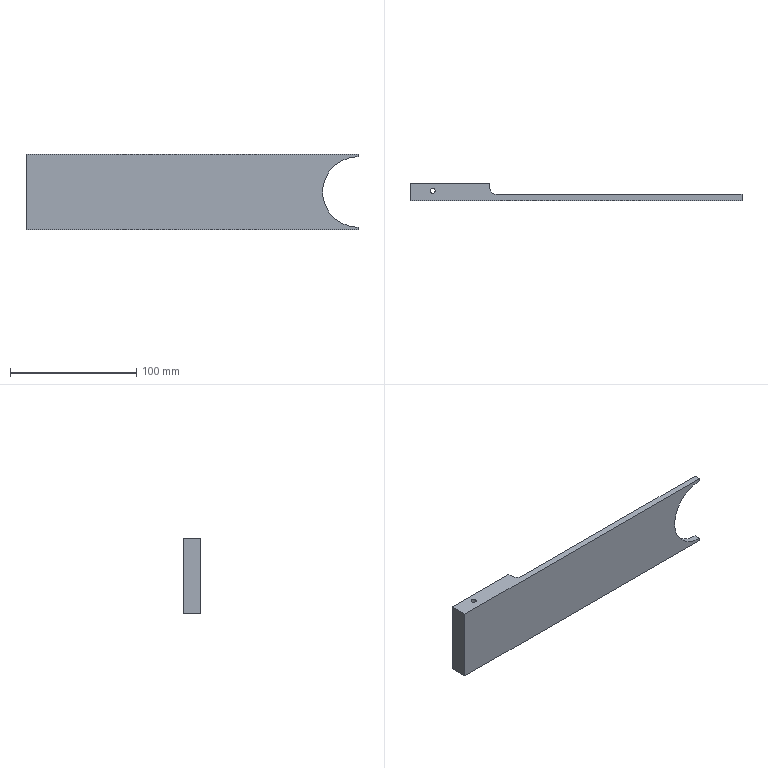Part | SolidWorks | features ICE 2, Extrusion 1, Fillet 1 | 1 solid | 13 faces | box 263.439 x 13.991 x 60 mm | volume 106666 mm3 | plane 9 | cylinder 4 | commonest cylinder face diameters 4 x2 10 x1 56 x1
STEP:
#1=CARTESIAN_POINT('',(-97.439,5.491,-30.));
#2=VERTEX_POINT('',#1);
#3=CARTESIAN_POINT('',(-93.439,5.491,-30.));
#4=VERTEX_POINT('',#3);
#5=CARTESIAN_POINT('',(-95.439,5.491,-30.));
#6=DIRECTION('',(0.,0.,1.));
#7=DIRECTION('',(1.,0.,0.));
#8=AXIS2_PLACEMENT_3D('',#5,#6,#7);
#9=CIRCLE('',#8,2.);
#10=EDGE_CURVE('',#2,#4,#9,.T.);
#11=ORIENTED_EDGE('',*,*,#10,.F.);
#12=CARTESIAN_POINT('',(-97.439,5.491,30.));
#13=VERTEX_POINT('',#12);
#14=CARTESIAN_POINT('',(-97.439,5.491,-30.));
#15=DIRECTION('',(0.,0.,1.));
#16=VECTOR('',#15,1000.);
#17=LINE('',#14,#16);
#18=EDGE_CURVE('',#2,#13,#17,.T.);
#19=ORIENTED_EDGE('',*,*,#18,.T.);
#20=CARTESIAN_POINT('',(-93.439,5.491,30.));
#21=VERTEX_POINT('',#20);
#22=CARTESIAN_POINT('',(-95.439,5.491,30.));
#23=DIRECTION('',(0.,0.,1.));
#24=DIRECTION('',(1.,0.,0.));
#25=AXIS2_PLACEMENT_3D('',#22,#23,#24);
#26=CIRCLE('',#25,2.);
#27=EDGE_CURVE('',#13,#21,#26,.T.);
#28=ORIENTED_EDGE('',*,*,#27,.T.);
#29=CARTESIAN_POINT('',(-93.439,5.491,-30.));
#30=DIRECTION('',(0.,0.,1.));
#31=VECTOR('',#30,1000.);
#32=LINE('',#29,#31);
#33=EDGE_CURVE('',#4,#21,#32,.T.);
#34=ORIENTED_EDGE('',*,*,#33,.F.);
#35=EDGE_LOOP('',(#11,#19,#28,#34));
#36=FACE_OUTER_BOUND('',#35,.T.);
#37=CARTESIAN_POINT('',(-95.439,5.491,-30.));
#38=DIRECTION('',(0.,0.,1.));
#39=DIRECTION('',(1.,0.,0.));
#40=AXIS2_PLACEMENT_3D('',#37,#38,#39);
#41=CYLINDRICAL_SURFACE('',#40,2.);
#42=ADVANCED_FACE('',(#36),#41,.F.);
#43=CARTESIAN_POINT('',(150.,-2.5,30.));
#44=VERTEX_POINT('',#43);
#45=CARTESIAN_POINT('',(150.,-2.5,28.));
#46=VERTEX_POINT('',#45);
#47=CARTESIAN_POINT('',(150.,-2.5,30.));
#48=DIRECTION('',(0.,0.,-1.));
#49=VECTOR('',#48,1000.);
#50=LINE('',#47,#49);
#51=EDGE_CURVE('',#44,#46,#50,.T.);
#52=ORIENTED_EDGE('',*,*,#51,.T.);
#53=CARTESIAN_POINT('',(150.,2.5,28.));
#54=VERTEX_POINT('',#53);
#55=CARTESIAN_POINT('',(150.,2.5,28.));
#56=DIRECTION('',(0.,-1.,0.));
#57=VECTOR('',#56,1000.);
#58=LINE('',#55,#57);
#59=EDGE_CURVE('',#54,#46,#58,.T.);
#60=ORIENTED_EDGE('',*,*,#59,.F.);
#61=CARTESIAN_POINT('',(150.,2.5,30.));
#62=VERTEX_POINT('',#61);
#63=CARTESIAN_POINT('',(150.,2.5,30.));
#64=DIRECTION('',(0.,0.,-1.));
#65=VECTOR('',#64,1000.);
#66=LINE('',#63,#65);
#67=EDGE_CURVE('',#62,#54,#66,.T.);
#68=ORIENTED_EDGE('',*,*,#67,.F.);
#69=CARTESIAN_POINT('',(150.,2.5,30.));
#70=DIRECTION('',(0.,-1.,0.));
#71=VECTOR('',#70,1000.);
#72=LINE('',#69,#71);
#73=EDGE_CURVE('',#62,#44,#72,.T.);
#74=ORIENTED_EDGE('',*,*,#73,.T.);
#75=EDGE_LOOP('',(#52,#60,#68,#74));
#76=FACE_OUTER_BOUND('',#75,.T.);
#77=CARTESIAN_POINT('',(150.,2.5,30.));
#78=DIRECTION('',(-1.,0.,0.));
#79=DIRECTION('',(0.,0.,1.));
#80=AXIS2_PLACEMENT_3D('',#77,#78,#79);
#81=PLANE('',#80);
#82=ADVANCED_FACE('',(#76),#81,.F.);
#83=CARTESIAN_POINT('',(150.,-2.5,-28.));
#84=VERTEX_POINT('',#83);
#85=CARTESIAN_POINT('',(150.,-2.5,0.));
#86=DIRECTION('',(0.,-1.,0.));
#87=DIRECTION('',(0.,0.,1.));
#88=AXIS2_PLACEMENT_3D('',#85,#86,#87);
#89=CIRCLE('',#88,28.);
#90=EDGE_CURVE('',#46,#84,#89,.T.);
#91=ORIENTED_EDGE('',*,*,#90,.T.);
#92=CARTESIAN_POINT('',(150.,2.5,-28.));
#93=VERTEX_POINT('',#92);
#94=CARTESIAN_POINT('',(150.,2.5,-28.));
#95=DIRECTION('',(0.,-1.,0.));
#96=VECTOR('',#95,1000.);
#97=LINE('',#94,#96);
#98=EDGE_CURVE('',#93,#84,#97,.T.);
#99=ORIENTED_EDGE('',*,*,#98,.F.);
#100=CARTESIAN_POINT('',(150.,2.5,0.));
#101=DIRECTION('',(0.,-1.,0.));
#102=DIRECTION('',(0.,0.,1.));
#103=AXIS2_PLACEMENT_3D('',#100,#101,#102);
#104=CIRCLE('',#103,28.);
#105=EDGE_CURVE('',#54,#93,#104,.T.);
#106=ORIENTED_EDGE('',*,*,#105,.F.);
#107=ORIENTED_EDGE('',*,*,#59,.T.);
#108=EDGE_LOOP('',(#91,#99,#106,#107));
#109=FACE_OUTER_BOUND('',#108,.T.);
#110=CARTESIAN_POINT('',(150.,2.5,0.));
#111=DIRECTION('',(0.,-1.,0.));
#112=DIRECTION('',(0.,0.,-1.));
#113=AXIS2_PLACEMENT_3D('',#110,#111,#112);
#114=CYLINDRICAL_SURFACE('',#113,28.);
#115=ADVANCED_FACE('',(#109),#114,.F.);
#116=CARTESIAN_POINT('',(150.,-2.5,-30.));
#117=VERTEX_POINT('',#116);
#118=CARTESIAN_POINT('',(150.,-2.5,-28.));
#119=DIRECTION('',(0.,0.,-1.));
#120=VECTOR('',#119,1000.);
#121=LINE('',#118,#120);
#122=EDGE_CURVE('',#84,#117,#121,.T.);
#123=ORIENTED_EDGE('',*,*,#122,.T.);
#124=CARTESIAN_POINT('',(150.,2.5,-30.));
#125=VERTEX_POINT('',#124);
#126=CARTESIAN_POINT('',(150.,2.5,-30.));
#127=DIRECTION('',(0.,-1.,0.));
#128=VECTOR('',#127,1000.);
#129=LINE('',#126,#128);
#130=EDGE_CURVE('',#125,#117,#129,.T.);
#131=ORIENTED_EDGE('',*,*,#130,.F.);
#132=CARTESIAN_POINT('',(150.,2.5,-28.));
#133=DIRECTION('',(0.,0.,-1.));
#134=VECTOR('',#133,1000.);
#135=LINE('',#132,#134);
#136=EDGE_CURVE('',#93,#125,#135,.T.);
#137=ORIENTED_EDGE('',*,*,#136,.F.);
#138=ORIENTED_EDGE('',*,*,#98,.T.);
#139=EDGE_LOOP('',(#123,#131,#137,#138));
#140=FACE_OUTER_BOUND('',#139,.T.);
#141=CARTESIAN_POINT('',(150.,2.5,-28.));
#142=DIRECTION('',(-1.,0.,0.));
#143=DIRECTION('',(0.,0.,1.));
#144=AXIS2_PLACEMENT_3D('',#141,#142,#143);
#145=PLANE('',#144);
#146=ADVANCED_FACE('',(#140),#145,.F.);
#147=CARTESIAN_POINT('',(-95.439,5.491,-30.));
#148=DIRECTION('',(0.,0.,1.));
#149=DIRECTION('',(1.,0.,0.));
#150=AXIS2_PLACEMENT_3D('',#147,#148,#149);
#151=CIRCLE('',#150,2.);
#152=EDGE_CURVE('',#4,#2,#151,.T.);
#153=ORIENTED_EDGE('',*,*,#152,.T.);
#154=ORIENTED_EDGE('',*,*,#10,.T.);
#155=EDGE_LOOP('',(#153,#154));
#156=FACE_BOUND('',#155,.T.);
#157=CARTESIAN_POINT('',(-113.439,-2.5,-30.));
#158=VERTEX_POINT('',#157);
#159=CARTESIAN_POINT('',(-50.,-2.5,-30.));
#160=DIRECTION('',(-1.,0.,0.));
#161=VECTOR('',#160,1000.);
#162=LINE('',#159,#161);
#163=EDGE_CURVE('',#117,#158,#162,.T.);
#164=ORIENTED_EDGE('',*,*,#163,.T.);
#165=CARTESIAN_POINT('',(-113.439,11.491,-30.));
#166=VERTEX_POINT('',#165);
#167=CARTESIAN_POINT('',(-113.439,-2.5,-30.));
#168=DIRECTION('',(0.,-1.,0.));
#169=VECTOR('',#168,1000.);
#170=LINE('',#167,#169);
#171=EDGE_CURVE('',#166,#158,#170,.T.);
#172=ORIENTED_EDGE('',*,*,#171,.F.);
#173=CARTESIAN_POINT('',(-50.,11.491,-30.));
#174=VERTEX_POINT('',#173);
#175=CARTESIAN_POINT('',(-50.,11.491,-30.));
#176=DIRECTION('',(-1.,0.,0.));
#177=VECTOR('',#176,1000.);
#178=LINE('',#175,#177);
#179=EDGE_CURVE('',#174,#166,#178,.T.);
#180=ORIENTED_EDGE('',*,*,#179,.F.);
#181=CARTESIAN_POINT('',(-50.,7.5,-30.));
#182=VERTEX_POINT('',#181);
#183=CARTESIAN_POINT('',(-50.,-2.5,-30.));
#184=DIRECTION('',(0.,1.,0.));
#185=VECTOR('',#184,1000.);
#186=LINE('',#183,#185);
#187=EDGE_CURVE('',#182,#174,#186,.T.);
#188=ORIENTED_EDGE('',*,*,#187,.F.);
#189=CARTESIAN_POINT('',(-45.,2.5,-30.));
#190=VERTEX_POINT('',#189);
#191=CARTESIAN_POINT('',(-45.,7.5,-30.));
#192=DIRECTION('',(0.,0.,1.));
#193=DIRECTION('',(1.,0.,0.));
#194=AXIS2_PLACEMENT_3D('',#191,#192,#193);
#195=CIRCLE('',#194,5.);
#196=EDGE_CURVE('',#182,#190,#195,.T.);
#197=ORIENTED_EDGE('',*,*,#196,.T.);
#198=CARTESIAN_POINT('',(150.,2.5,-30.));
#199=DIRECTION('',(-1.,0.,0.));
#200=VECTOR('',#199,1000.);
#201=LINE('',#198,#200);
#202=EDGE_CURVE('',#125,#190,#201,.T.);
#203=ORIENTED_EDGE('',*,*,#202,.F.);
#204=ORIENTED_EDGE('',*,*,#130,.T.);
#205=EDGE_LOOP('',(#164,#172,#180,#188,#197,#203,#204));
#206=FACE_OUTER_BOUND('',#205,.T.);
#207=CARTESIAN_POINT('',(-50.,2.5,-30.));
#208=DIRECTION('',(0.,0.,1.));
#209=DIRECTION('',(1.,0.,0.));
#210=AXIS2_PLACEMENT_3D('',#207,#208,#209);
#211=PLANE('',#210);
#212=ADVANCED_FACE('',(#156,#206),#211,.F.);
#213=CARTESIAN_POINT('',(-95.439,5.491,30.));
#214=DIRECTION('',(0.,0.,1.));
#215=DIRECTION('',(1.,0.,0.));
#216=AXIS2_PLACEMENT_3D('',#213,#214,#215);
#217=CIRCLE('',#216,2.);
#218=EDGE_CURVE('',#21,#13,#217,.T.);
#219=ORIENTED_EDGE('',*,*,#218,.F.);
#220=ORIENTED_EDGE('',*,*,#27,.F.);
#221=EDGE_LOOP('',(#219,#220));
#222=FACE_BOUND('',#221,.T.);
#223=CARTESIAN_POINT('',(-113.439,-2.5,30.));
#224=VERTEX_POINT('',#223);
#225=CARTESIAN_POINT('',(-50.,-2.5,30.));
#226=DIRECTION('',(1.,0.,0.));
#227=VECTOR('',#226,1000.);
#228=LINE('',#225,#227);
#229=EDGE_CURVE('',#224,#44,#228,.T.);
#230=ORIENTED_EDGE('',*,*,#229,.T.);
#231=ORIENTED_EDGE('',*,*,#73,.F.);
#232=CARTESIAN_POINT('',(-45.,2.5,30.));
#233=VERTEX_POINT('',#232);
#234=CARTESIAN_POINT('',(50.,2.5,30.));
#235=DIRECTION('',(1.,0.,0.));
#236=VECTOR('',#235,1000.);
#237=LINE('',#234,#236);
#238=EDGE_CURVE('',#233,#62,#237,.T.);
#239=ORIENTED_EDGE('',*,*,#238,.F.);
#240=CARTESIAN_POINT('',(-50.,7.5,30.));
#241=VERTEX_POINT('',#240);
#242=CARTESIAN_POINT('',(-45.,7.5,30.));
#243=DIRECTION('',(0.,0.,-1.));
#244=DIRECTION('',(-1.,0.,0.));
#245=AXIS2_PLACEMENT_3D('',#242,#243,#244);
#246=CIRCLE('',#245,5.);
#247=EDGE_CURVE('',#233,#241,#246,.T.);
#248=ORIENTED_EDGE('',*,*,#247,.T.);
#249=CARTESIAN_POINT('',(-50.,11.491,30.));
#250=VERTEX_POINT('',#249);
#251=CARTESIAN_POINT('',(-50.,-2.5,30.));
#252=DIRECTION('',(0.,1.,0.));
#253=VECTOR('',#252,1000.);
#254=LINE('',#251,#253);
#255=EDGE_CURVE('',#241,#250,#254,.T.);
#256=ORIENTED_EDGE('',*,*,#255,.T.);
#257=CARTESIAN_POINT('',(-113.439,11.491,30.));
#258=VERTEX_POINT('',#257);
#259=CARTESIAN_POINT('',(-50.,11.491,30.));
#260=DIRECTION('',(-1.,0.,0.));
#261=VECTOR('',#260,1000.);
#262=LINE('',#259,#261);
#263=EDGE_CURVE('',#250,#258,#262,.T.);
#264=ORIENTED_EDGE('',*,*,#263,.T.);
#265=CARTESIAN_POINT('',(-113.439,-2.5,30.));
#266=DIRECTION('',(0.,-1.,0.));
#267=VECTOR('',#266,1000.);
#268=LINE('',#265,#267);
#269=EDGE_CURVE('',#258,#224,#268,.T.);
#270=ORIENTED_EDGE('',*,*,#269,.T.);
#271=EDGE_LOOP('',(#230,#231,#239,#248,#256,#264,#270));
#272=FACE_OUTER_BOUND('',#271,.T.);
#273=CARTESIAN_POINT('',(-50.,2.5,30.));
#274=DIRECTION('',(0.,0.,-1.));
#275=DIRECTION('',(-1.,0.,0.));
#276=AXIS2_PLACEMENT_3D('',#273,#274,#275);
#277=PLANE('',#276);
#278=ADVANCED_FACE('',(#222,#272),#277,.F.);
#279=ORIENTED_EDGE('',*,*,#202,.T.);
#280=CARTESIAN_POINT('',(-45.,2.5,0.));
#281=DIRECTION('',(0.,0.,1.));
#282=VECTOR('',#281,1000.);
#283=LINE('',#280,#282);
#284=EDGE_CURVE('',#190,#233,#283,.T.);
#285=ORIENTED_EDGE('',*,*,#284,.T.);
#286=ORIENTED_EDGE('',*,*,#238,.T.);
#287=ORIENTED_EDGE('',*,*,#67,.T.);
#288=ORIENTED_EDGE('',*,*,#105,.T.);
#289=ORIENTED_EDGE('',*,*,#136,.T.);
#290=EDGE_LOOP('',(#279,#285,#286,#287,#288,#289));
#291=FACE_OUTER_BOUND('',#290,.T.);
#292=CARTESIAN_POINT('',(150.,2.5,0.));
#293=DIRECTION('',(0.,1.,0.));
#294=DIRECTION('',(0.,0.,1.));
#295=AXIS2_PLACEMENT_3D('',#292,#293,#294);
#296=PLANE('',#295);
#297=ADVANCED_FACE('',(#291),#296,.T.);
#298=ORIENTED_EDGE('',*,*,#51,.F.);
#299=ORIENTED_EDGE('',*,*,#229,.F.);
#300=CARTESIAN_POINT('',(-113.439,-2.5,30.));
#301=DIRECTION('',(0.,0.,-1.));
#302=VECTOR('',#301,1000.);
#303=LINE('',#300,#302);
#304=EDGE_CURVE('',#224,#158,#303,.T.);
#305=ORIENTED_EDGE('',*,*,#304,.T.);
#306=ORIENTED_EDGE('',*,*,#163,.F.);
#307=ORIENTED_EDGE('',*,*,#122,.F.);
#308=ORIENTED_EDGE('',*,*,#90,.F.);
#309=EDGE_LOOP('',(#298,#299,#305,#306,#307,#308));
#310=FACE_OUTER_BOUND('',#309,.T.);
#311=CARTESIAN_POINT('',(150.,-2.5,0.));
#312=DIRECTION('',(0.,1.,0.));
#313=DIRECTION('',(0.,0.,1.));
#314=AXIS2_PLACEMENT_3D('',#311,#312,#313);
#315=PLANE('',#314);
#316=ADVANCED_FACE('',(#310),#315,.F.);
#317=ORIENTED_EDGE('',*,*,#255,.F.);
#318=CARTESIAN_POINT('',(-50.,7.5,30.));
#319=DIRECTION('',(0.,0.,-1.));
#320=VECTOR('',#319,1000.);
#321=LINE('',#318,#320);
#322=EDGE_CURVE('',#241,#182,#321,.T.);
#323=ORIENTED_EDGE('',*,*,#322,.T.);
#324=ORIENTED_EDGE('',*,*,#187,.T.);
#325=CARTESIAN_POINT('',(-50.,11.491,30.));
#326=DIRECTION('',(0.,0.,-1.));
#327=VECTOR('',#326,1000.);
#328=LINE('',#325,#327);
#329=EDGE_CURVE('',#250,#174,#328,.T.);
#330=ORIENTED_EDGE('',*,*,#329,.F.);
#331=EDGE_LOOP('',(#317,#323,#324,#330));
#332=FACE_OUTER_BOUND('',#331,.T.);
#333=CARTESIAN_POINT('',(-50.,-2.5,30.));
#334=DIRECTION('',(-1.,0.,0.));
#335=DIRECTION('',(0.,0.,1.));
#336=AXIS2_PLACEMENT_3D('',#333,#334,#335);
#337=PLANE('',#336);
#338=ADVANCED_FACE('',(#332),#337,.F.);
#339=ORIENTED_EDGE('',*,*,#179,.T.);
#340=CARTESIAN_POINT('',(-113.439,11.491,30.));
#341=DIRECTION('',(0.,0.,-1.));
#342=VECTOR('',#341,1000.);
#343=LINE('',#340,#342);
#344=EDGE_CURVE('',#258,#166,#343,.T.);
#345=ORIENTED_EDGE('',*,*,#344,.F.);
#346=ORIENTED_EDGE('',*,*,#263,.F.);
#347=ORIENTED_EDGE('',*,*,#329,.T.);
#348=EDGE_LOOP('',(#339,#345,#346,#347));
#349=FACE_OUTER_BOUND('',#348,.T.);
#350=CARTESIAN_POINT('',(-50.,11.491,30.));
#351=DIRECTION('',(0.,-1.,0.));
#352=DIRECTION('',(1.,0.,0.));
#353=AXIS2_PLACEMENT_3D('',#350,#351,#352);
#354=PLANE('',#353);
#355=ADVANCED_FACE('',(#349),#354,.F.);
#356=ORIENTED_EDGE('',*,*,#171,.T.);
#357=ORIENTED_EDGE('',*,*,#304,.F.);
#358=ORIENTED_EDGE('',*,*,#269,.F.);
#359=ORIENTED_EDGE('',*,*,#344,.T.);
#360=EDGE_LOOP('',(#356,#357,#358,#359));
#361=FACE_OUTER_BOUND('',#360,.T.);
#362=CARTESIAN_POINT('',(-113.439,-2.5,30.));
#363=DIRECTION('',(1.,0.,0.));
#364=DIRECTION('',(0.,0.,-1.));
#365=AXIS2_PLACEMENT_3D('',#362,#363,#364);
#366=PLANE('',#365);
#367=ADVANCED_FACE('',(#361),#366,.F.);
#368=ORIENTED_EDGE('',*,*,#196,.F.);
#369=ORIENTED_EDGE('',*,*,#322,.F.);
#370=ORIENTED_EDGE('',*,*,#247,.F.);
#371=ORIENTED_EDGE('',*,*,#284,.F.);
#372=EDGE_LOOP('',(#368,#369,#370,#371));
#373=FACE_OUTER_BOUND('',#372,.T.);
#374=CARTESIAN_POINT('',(-45.,7.5,0.));
#375=DIRECTION('',(0.,0.,1.));
#376=DIRECTION('',(1.,0.,0.));
#377=AXIS2_PLACEMENT_3D('',#374,#375,#376);
#378=CYLINDRICAL_SURFACE('',#377,5.);
#379=ADVANCED_FACE('',(#373),#378,.F.);
#380=ORIENTED_EDGE('',*,*,#18,.F.);
#381=ORIENTED_EDGE('',*,*,#152,.F.);
#382=ORIENTED_EDGE('',*,*,#33,.T.);
#383=ORIENTED_EDGE('',*,*,#218,.T.);
#384=EDGE_LOOP('',(#380,#381,#382,#383));
#385=FACE_OUTER_BOUND('',#384,.T.);
#386=CARTESIAN_POINT('',(-95.439,5.491,-30.));
#387=DIRECTION('',(0.,0.,1.));
#388=DIRECTION('',(1.,0.,0.));
#389=AXIS2_PLACEMENT_3D('',#386,#387,#388);
#390=CYLINDRICAL_SURFACE('',#389,2.);
#391=ADVANCED_FACE('',(#385),#390,.F.);
#392=CLOSED_SHELL('',(#42,#82,#115,#146,#212,#278,#297,#316,#338,#355,#367,#379,#391));
#393=MANIFOLD_SOLID_BREP('',#392);
#394=CARTESIAN_POINT('',(0.,0.,0.));
#395=DIRECTION('',(0.,0.,1.));
#396=DIRECTION('',(1.,0.,0.));
#397=AXIS2_PLACEMENT_3D('',#394,#395,#396);
#398=(LENGTH_UNIT()NAMED_UNIT(*)SI_UNIT(.MILLI.,.METRE.));
#399=UNCERTAINTY_MEASURE_WITH_UNIT(LENGTH_MEASURE(0.00001),#398,'','');
#400=(NAMED_UNIT(*)PLANE_ANGLE_UNIT()SI_UNIT($,.RADIAN.));
#401=(NAMED_UNIT(*)SI_UNIT($,.STERADIAN.)SOLID_ANGLE_UNIT());
#402=(GEOMETRIC_REPRESENTATION_CONTEXT(3)GLOBAL_UNCERTAINTY_ASSIGNED_CONTEXT((#399))GLOBAL_UNIT_ASSIGNED_CONTEXT((#398,#400,#401))REPRESENTATION_CONTEXT('',''));
#403=ADVANCED_BREP_SHAPE_REPRESENTATION('',(#393,#397),#402);